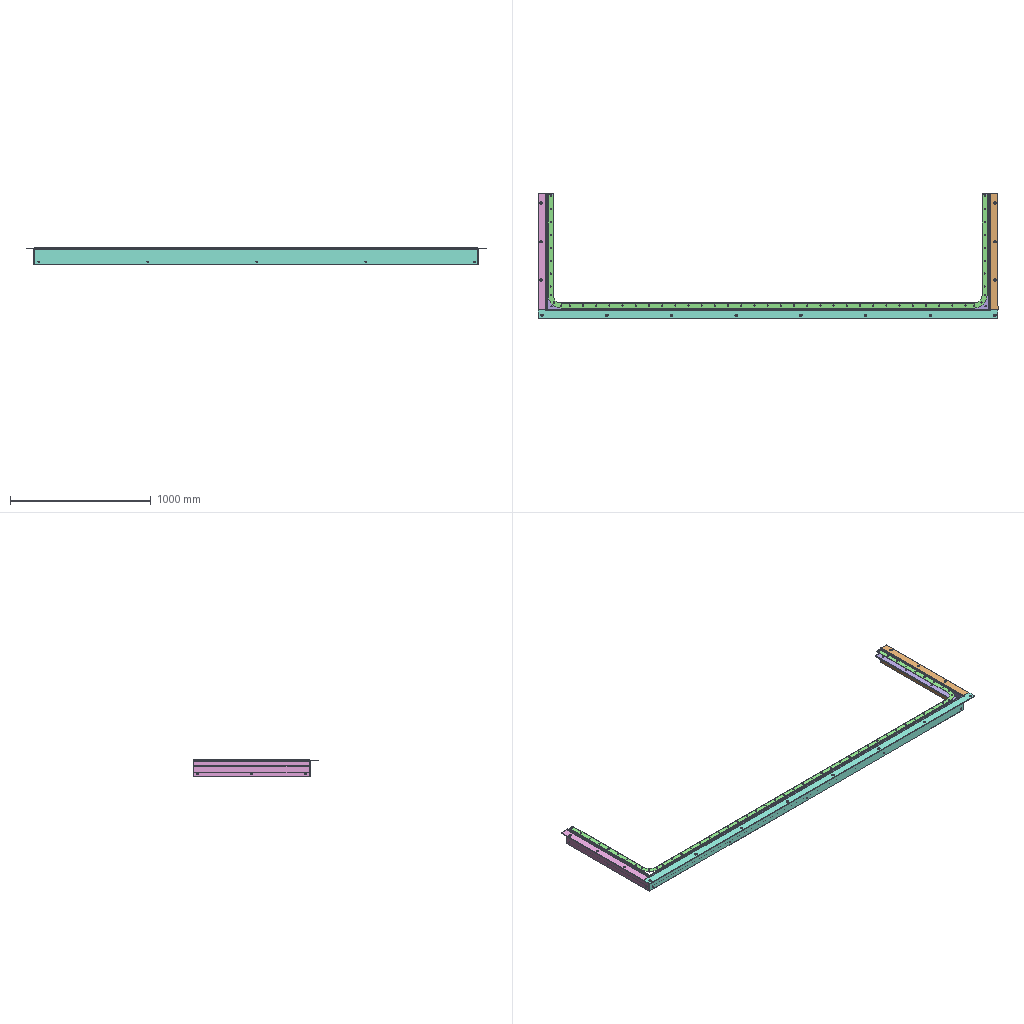Assembly | SolidWorks | 15 different items | 82 placed | box 3271 x 887 x 127 mm
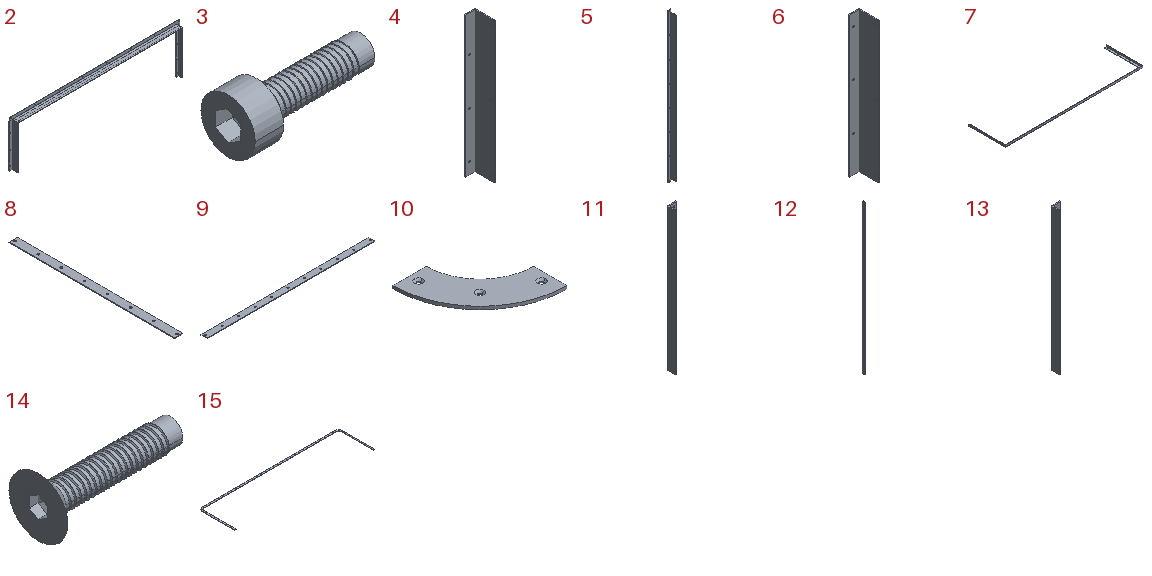Parts list (item | name | quantity | parent item | size | volume | features):
1 | 10 window threaded screw alignment | x1 | - | - | - | -
2 | (subassembly) | x1 | - | 3271 x 120 x 887 mm | 7624101 mm3 | -
3 | - | x16 | - | 31.8 x 13 x 13 mm | 1679 mm3 | features BlendCut 1, ICE 1, Revolution 1, SweepThread 1
4 | - | x1 | in 2 | 60 x 120 x 827 mm | 851995 mm3 | features BaseBody 1
5 | - | x1 | in 2 | 60 x 120 x 3271 mm | 3298320 mm3 | features BaseBody 1
6 | - | x1 | in 2 | 60 x 120 x 827 mm | 851995 mm3 | features BaseBody 1
7 | - | x1 | - | 3151 x 827 x 44 mm | 1704448 mm3 | features BaseBody 1
8 | - | x1 | - | 35 x 712 x 3.2 mm | 79027 mm3 | features BaseBody 1
9 | - | x1 | - | 979 x 35 x 3.2 mm | 108662 mm3 | features BaseBody 1
10 | - | x1 | - | 92 x 92 x 3.2 mm | 12838 mm3 | features BaseBody 1
11 | - | x1 | in 2 | 50 x 50 x 821 mm | 453617 mm3 | features BaseBody 1
12 | - | x1 | in 2 | 50 x 50 x 3151 mm | 1714556 mm3 | features BaseBody 1
13 | - | x1 | in 2 | 50 x 50 x 821 mm | 453617 mm3 | features BaseBody 1
14 | - | x53 | - | 18.05 x 8 x 8 mm | 188.407 mm3 | features BlendCut 1, ICE 1, Revolution 1, SweepThread 1
15 | - | x1 | - | 3121 x 804 x 3 mm | 477899 mm3 | features ICE 3, Extrusion 1
Mates (type | each side: item.copy, entity, surface, feature):
DistanceDim | 15.1 face plane Boss-Extrude1 | 7.1 face plane Input1
Coincident | 15.1 face plane Boss-Extrude1 | 14.1 edge
Coincident | 15.1 face plane Boss-Extrude1 | 14.2 edge
Concentric | 15.1 edge | 14.2 edge
Coincident | 15.1 face plane Boss-Extrude1 | 14.3 edge
Concentric | 15.1 edge | 14.3 edge
Concentric | 15.1 edge | 14.4 edge
Coincident | 15.1 face plane Boss-Extrude1 | 14.4 edge
Coincident | 15.1 face plane Boss-Extrude1 | 14.5 edge
Concentric | 15.1 edge | 14.5 edge
Concentric | 11.1 face cylinder Input1 | 3.1 face cylinder Revolve1
Coincident | 11.1 face plane Input1 | 3.1 face plane Revolve1
Concentric | 11.1 edge | 3.2 edge
Coincident | 11.1 face plane Input1 | 3.2 edge
Concentric | 11.1 face cylinder Input1 | 3.3 face cylinder Revolve1
Coincident | 11.1 face plane Input1 | 3.3 edge
Coincident | 11.1 face plane Input1 | 3.4 edge
Concentric | 11.1 edge | 3.4 face cylinder Revolve1
Concentric | 12.1 face cylinder Input1 | 3.5 face cylinder Revolve1
Coincident | 12.1 face plane Input1 | 3.5 edge
Concentric | 13.1 face cylinder Input1 | 3.6 edge
Coincident | 13.1 face plane Input1 | 3.6 edge
Concentric | 13.1 edge | 3.7 edge
Coincident | 13.1 face plane Input1 | 3.7 edge
Coincident | 13.1 face plane Input1 | 3.8 edge
Concentric | 13.1 face cylinder Input1 | 3.8 face cylinder Revolve1
Coincident | 13.1 face plane Input1 | 3.9 edge
Concentric | 13.1 face cylinder Input1 | 3.9 face cylinder Revolve1
Coincident | 15.1 face plane Boss-Extrude1 | 14.6 face plane Revolve1
Concentric | 15.1 edge | 14.6 edge
Coincident | 15.1 face plane Boss-Extrude1 | 14.7 edge
Concentric | 15.1 edge | 14.7 edge
Coincident | 15.1 face plane Boss-Extrude1 | 14.8 edge
Concentric | 15.1 edge | 14.8 edge
Coincident | 15.1 face plane Boss-Extrude1 | 14.9 edge
Concentric | 15.1 edge | 14.9 edge